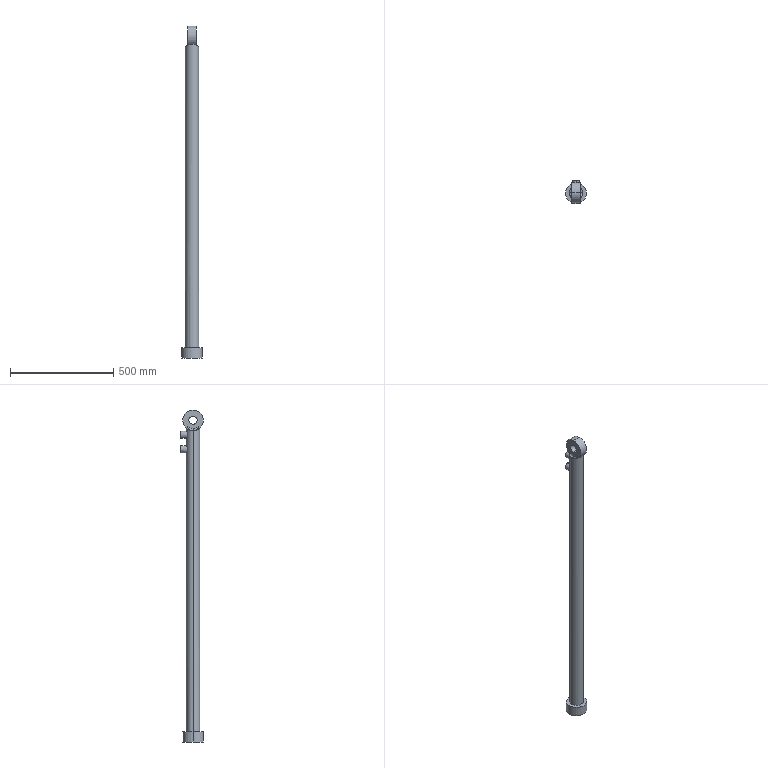Part | SolidWorks | features ICE 5, Fillet 2, Extrusion 1 | 1 solid | 30 faces | box 100 x 110 x 1610 mm | volume 5542883 mm3 | cylinder 18 | plane 8 | torus 4 | commonest cylinder face diameters 100 x6 20 x4 35 x4 40 x2 65 x2
STEP:
#1=CARTESIAN_POINT('',(0.,20.,1360.));
#2=VERTEX_POINT('',#1);
#3=CARTESIAN_POINT('',(0.,20.,1380.));
#4=VERTEX_POINT('',#3);
#5=CARTESIAN_POINT('',(0.,20.,1370.));
#6=DIRECTION('',(0.,1.,0.));
#7=DIRECTION('',(0.,0.,1.));
#8=AXIS2_PLACEMENT_3D('',#5,#6,#7);
#9=CIRCLE('',#8,10.);
#10=EDGE_CURVE('',#2,#4,#9,.T.);
#11=ORIENTED_EDGE('',*,*,#10,.F.);
#12=CARTESIAN_POINT('',(0.,60.,1360.));
#13=VERTEX_POINT('',#12);
#14=CARTESIAN_POINT('',(0.,20.,1360.));
#15=DIRECTION('',(0.,1.,0.));
#16=VECTOR('',#15,1000.);
#17=LINE('',#14,#16);
#18=EDGE_CURVE('',#2,#13,#17,.T.);
#19=ORIENTED_EDGE('',*,*,#18,.T.);
#20=CARTESIAN_POINT('',(0.,60.,1380.));
#21=VERTEX_POINT('',#20);
#22=CARTESIAN_POINT('',(0.,60.,1370.));
#23=DIRECTION('',(0.,1.,0.));
#24=DIRECTION('',(0.,0.,1.));
#25=AXIS2_PLACEMENT_3D('',#22,#23,#24);
#26=CIRCLE('',#25,10.);
#27=EDGE_CURVE('',#13,#21,#26,.T.);
#28=ORIENTED_EDGE('',*,*,#27,.T.);
#29=CARTESIAN_POINT('',(0.,20.,1380.));
#30=DIRECTION('',(0.,1.,0.));
#31=VECTOR('',#30,1000.);
#32=LINE('',#29,#31);
#33=EDGE_CURVE('',#4,#21,#32,.T.);
#34=ORIENTED_EDGE('',*,*,#33,.F.);
#35=EDGE_LOOP('',(#11,#19,#28,#34));
#36=FACE_OUTER_BOUND('',#35,.T.);
#37=CARTESIAN_POINT('',(0.,20.,1370.));
#38=DIRECTION('',(0.,1.,0.));
#39=DIRECTION('',(0.,0.,1.));
#40=AXIS2_PLACEMENT_3D('',#37,#38,#39);
#41=CYLINDRICAL_SURFACE('',#40,10.);
#42=ADVANCED_FACE('',(#36),#41,.F.);
#43=CARTESIAN_POINT('',(0.,20.,1430.));
#44=VERTEX_POINT('',#43);
#45=CARTESIAN_POINT('',(0.,20.,1450.));
#46=VERTEX_POINT('',#45);
#47=CARTESIAN_POINT('',(0.,20.,1440.));
#48=DIRECTION('',(0.,1.,0.));
#49=DIRECTION('',(0.,0.,1.));
#50=AXIS2_PLACEMENT_3D('',#47,#48,#49);
#51=CIRCLE('',#50,10.);
#52=EDGE_CURVE('',#44,#46,#51,.T.);
#53=ORIENTED_EDGE('',*,*,#52,.F.);
#54=CARTESIAN_POINT('',(0.,60.,1430.));
#55=VERTEX_POINT('',#54);
#56=CARTESIAN_POINT('',(0.,20.,1430.));
#57=DIRECTION('',(0.,1.,0.));
#58=VECTOR('',#57,1000.);
#59=LINE('',#56,#58);
#60=EDGE_CURVE('',#44,#55,#59,.T.);
#61=ORIENTED_EDGE('',*,*,#60,.T.);
#62=CARTESIAN_POINT('',(0.,60.,1450.));
#63=VERTEX_POINT('',#62);
#64=CARTESIAN_POINT('',(0.,60.,1440.));
#65=DIRECTION('',(0.,1.,0.));
#66=DIRECTION('',(0.,0.,1.));
#67=AXIS2_PLACEMENT_3D('',#64,#65,#66);
#68=CIRCLE('',#67,10.);
#69=EDGE_CURVE('',#55,#63,#68,.T.);
#70=ORIENTED_EDGE('',*,*,#69,.T.);
#71=CARTESIAN_POINT('',(0.,20.,1450.));
#72=DIRECTION('',(0.,1.,0.));
#73=VECTOR('',#72,1000.);
#74=LINE('',#71,#73);
#75=EDGE_CURVE('',#46,#63,#74,.T.);
#76=ORIENTED_EDGE('',*,*,#75,.F.);
#77=EDGE_LOOP('',(#53,#61,#70,#76));
#78=FACE_OUTER_BOUND('',#77,.T.);
#79=CARTESIAN_POINT('',(0.,20.,1440.));
#80=DIRECTION('',(0.,1.,0.));
#81=DIRECTION('',(0.,0.,1.));
#82=AXIS2_PLACEMENT_3D('',#79,#80,#81);
#83=CYLINDRICAL_SURFACE('',#82,10.);
#84=ADVANCED_FACE('',(#78),#83,.F.);
#85=CARTESIAN_POINT('',(0.,32.5,1387.5));
#86=VERTEX_POINT('',#85);
#87=CARTESIAN_POINT('',(0.,32.5,1352.5));
#88=VERTEX_POINT('',#87);
#89=CARTESIAN_POINT('',(0.,32.5,1387.5));
#90=CARTESIAN_POINT('',(1.182,32.5,1387.5));
#91=CARTESIAN_POINT('',(2.339,32.436,1387.382));
#92=CARTESIAN_POINT('',(4.042,32.253,1387.037));
#93=CARTESIAN_POINT('',(4.604,32.177,1386.893));
#94=CARTESIAN_POINT('',(5.717,31.998,1386.55));
#95=CARTESIAN_POINT('',(6.262,31.896,1386.351));
#96=CARTESIAN_POINT('',(7.847,31.557,1385.684));
#97=CARTESIAN_POINT('',(8.845,31.289,1385.143));
#98=CARTESIAN_POINT('',(10.259,30.842,1384.189));
#99=CARTESIAN_POINT('',(10.715,30.686,1383.848));
#100=CARTESIAN_POINT('',(11.583,30.369,1383.13));
#101=CARTESIAN_POINT('',(11.997,30.208,1382.753));
#102=CARTESIAN_POINT('',(12.787,29.882,1381.961));
#103=CARTESIAN_POINT('',(13.163,29.718,1381.545));
#104=CARTESIAN_POINT('',(13.878,29.391,1380.676));
#105=CARTESIAN_POINT('',(14.217,29.227,1380.22));
#106=CARTESIAN_POINT('',(15.16,28.756,1378.814));
#107=CARTESIAN_POINT('',(15.695,28.464,1377.824));
#108=CARTESIAN_POINT('',(16.354,28.086,1376.253));
#109=CARTESIAN_POINT('',(16.551,27.971,1375.715));
#110=CARTESIAN_POINT('',(16.807,27.817,1374.884));
#111=CARTESIAN_POINT('',(16.886,27.769,1374.603));
#112=CARTESIAN_POINT('',(17.03,27.681,1374.041));
#113=CARTESIAN_POINT('',(17.094,27.641,1373.758));
#114=CARTESIAN_POINT('',(17.381,27.463,1372.341));
#115=CARTESIAN_POINT('',(17.499,27.387,1371.19));
#116=CARTESIAN_POINT('',(17.501,27.386,1369.437));
#117=CARTESIAN_POINT('',(17.472,27.404,1368.843));
#118=CARTESIAN_POINT('',(17.355,27.478,1367.677));
#119=CARTESIAN_POINT('',(17.268,27.533,1367.102));
#120=CARTESIAN_POINT('',(17.039,27.676,1365.967));
#121=CARTESIAN_POINT('',(16.897,27.763,1365.408));
#122=CARTESIAN_POINT('',(16.557,27.967,1364.303));
#123=CARTESIAN_POINT('',(16.358,28.084,1363.757));
#124=CARTESIAN_POINT('',(15.693,28.465,1362.171));
#125=CARTESIAN_POINT('',(15.155,28.759,1361.177));
#126=CARTESIAN_POINT('',(14.208,29.232,1359.768));
#127=CARTESIAN_POINT('',(13.868,29.395,1359.312));
#128=CARTESIAN_POINT('',(13.153,29.722,1358.442));
#129=CARTESIAN_POINT('',(12.776,29.887,1358.028));
#130=CARTESIAN_POINT('',(11.985,30.213,1357.236));
#131=CARTESIAN_POINT('',(11.57,30.374,1356.859));
#132=CARTESIAN_POINT('',(10.702,30.691,1356.142));
#133=CARTESIAN_POINT('',(10.247,30.846,1355.802));
#134=CARTESIAN_POINT('',(8.828,31.294,1354.847));
#135=CARTESIAN_POINT('',(7.831,31.561,1354.308));
#136=CARTESIAN_POINT('',(6.255,31.897,1353.646));
#137=CARTESIAN_POINT('',(5.716,31.998,1353.45));
#138=CARTESIAN_POINT('',(4.609,32.176,1353.108));
#139=CARTESIAN_POINT('',(4.038,32.253,1352.962));
#140=CARTESIAN_POINT('',(2.323,32.437,1352.616));
#141=CARTESIAN_POINT('',(1.168,32.5,1352.5));
#142=CARTESIAN_POINT('',(0.,32.5,1352.5));
#143=B_SPLINE_CURVE_WITH_KNOTS('',3,(#89,#90,#91,#92,#93,#94,#95,#96,#97,#98,#99,#100,#101,#102,#103,#104,#105,#106,#107,#108,#109,#110,#111,#112,#113,#114,#115,#116,#117,#118,#119,#120,#121,#122,#123,#124,#125,#126,#127,#128,#129,#130,#131,#132,#133,#134,#135,#136,#137,#138,#139,#140,#141,#142),.UNSPECIFIED.,.F.,.F.,(4,2,2,2,2,2,2,2,2,2,2,2,2,2,2,2,2,2,2,2,2,2,2,2,2,2,4),(0.,0.00349,0.005235,0.00698,0.01047,0.01222,0.01396,0.01571,0.01745,0.02094,0.02269,0.02356,0.02443,0.02792,0.02967,0.03141,0.03316,0.0349,0.03839,0.04014,0.04188,0.04363,0.04537,0.04886,0.05061,0.05235,0.05584),.UNSPECIFIED.);
#144=EDGE_CURVE('',#86,#88,#143,.T.);
#145=ORIENTED_EDGE('',*,*,#144,.T.);
#146=CARTESIAN_POINT('',(0.,60.,1352.5));
#147=VERTEX_POINT('',#146);
#148=CARTESIAN_POINT('',(0.,-50.001,1352.5));
#149=DIRECTION('',(0.,1.,0.));
#150=VECTOR('',#149,1000.);
#151=LINE('',#148,#150);
#152=EDGE_CURVE('',#88,#147,#151,.T.);
#153=ORIENTED_EDGE('',*,*,#152,.T.);
#154=CARTESIAN_POINT('',(0.,60.,1387.5));
#155=VERTEX_POINT('',#154);
#156=CARTESIAN_POINT('',(0.,60.,1370.));
#157=DIRECTION('',(0.,1.,0.));
#158=DIRECTION('',(0.,0.,1.));
#159=AXIS2_PLACEMENT_3D('',#156,#157,#158);
#160=CIRCLE('',#159,17.5);
#161=EDGE_CURVE('',#155,#147,#160,.T.);
#162=ORIENTED_EDGE('',*,*,#161,.F.);
#163=CARTESIAN_POINT('',(0.,-50.001,1387.5));
#164=DIRECTION('',(0.,1.,0.));
#165=VECTOR('',#164,1000.);
#166=LINE('',#163,#165);
#167=EDGE_CURVE('',#86,#155,#166,.T.);
#168=ORIENTED_EDGE('',*,*,#167,.F.);
#169=EDGE_LOOP('',(#145,#153,#162,#168));
#170=FACE_OUTER_BOUND('',#169,.T.);
#171=CARTESIAN_POINT('',(0.,-50.001,1370.));
#172=DIRECTION('',(0.,1.,0.));
#173=DIRECTION('',(0.,0.,1.));
#174=AXIS2_PLACEMENT_3D('',#171,#172,#173);
#175=CYLINDRICAL_SURFACE('',#174,17.5);
#176=ADVANCED_FACE('',(#170),#175,.T.);
#177=CARTESIAN_POINT('',(0.,32.5,1457.5));
#178=VERTEX_POINT('',#177);
#179=CARTESIAN_POINT('',(0.,32.5,1422.5));
#180=VERTEX_POINT('',#179);
#181=CARTESIAN_POINT('',(0.,32.5,1457.5));
#182=CARTESIAN_POINT('',(1.182,32.5,1457.5));
#183=CARTESIAN_POINT('',(2.339,32.436,1457.382));
#184=CARTESIAN_POINT('',(4.042,32.253,1457.037));
#185=CARTESIAN_POINT('',(4.604,32.177,1456.893));
#186=CARTESIAN_POINT('',(5.717,31.998,1456.55));
#187=CARTESIAN_POINT('',(6.262,31.896,1456.351));
#188=CARTESIAN_POINT('',(7.847,31.557,1455.684));
#189=CARTESIAN_POINT('',(8.845,31.289,1455.143));
#190=CARTESIAN_POINT('',(10.259,30.842,1454.189));
#191=CARTESIAN_POINT('',(10.715,30.686,1453.848));
#192=CARTESIAN_POINT('',(11.583,30.369,1453.13));
#193=CARTESIAN_POINT('',(11.997,30.208,1452.753));
#194=CARTESIAN_POINT('',(12.787,29.882,1451.961));
#195=CARTESIAN_POINT('',(13.163,29.718,1451.545));
#196=CARTESIAN_POINT('',(13.878,29.391,1450.676));
#197=CARTESIAN_POINT('',(14.217,29.227,1450.22));
#198=CARTESIAN_POINT('',(15.16,28.756,1448.814));
#199=CARTESIAN_POINT('',(15.695,28.464,1447.824));
#200=CARTESIAN_POINT('',(16.354,28.086,1446.253));
#201=CARTESIAN_POINT('',(16.551,27.971,1445.715));
#202=CARTESIAN_POINT('',(16.807,27.817,1444.884));
#203=CARTESIAN_POINT('',(16.886,27.769,1444.603));
#204=CARTESIAN_POINT('',(17.03,27.681,1444.041));
#205=CARTESIAN_POINT('',(17.094,27.641,1443.758));
#206=CARTESIAN_POINT('',(17.381,27.463,1442.341));
#207=CARTESIAN_POINT('',(17.499,27.387,1441.19));
#208=CARTESIAN_POINT('',(17.501,27.386,1439.437));
#209=CARTESIAN_POINT('',(17.472,27.404,1438.843));
#210=CARTESIAN_POINT('',(17.355,27.478,1437.677));
#211=CARTESIAN_POINT('',(17.268,27.533,1437.102));
#212=CARTESIAN_POINT('',(17.039,27.676,1435.967));
#213=CARTESIAN_POINT('',(16.897,27.763,1435.408));
#214=CARTESIAN_POINT('',(16.557,27.967,1434.303));
#215=CARTESIAN_POINT('',(16.358,28.084,1433.757));
#216=CARTESIAN_POINT('',(15.693,28.465,1432.171));
#217=CARTESIAN_POINT('',(15.155,28.759,1431.177));
#218=CARTESIAN_POINT('',(14.208,29.232,1429.768));
#219=CARTESIAN_POINT('',(13.868,29.395,1429.312));
#220=CARTESIAN_POINT('',(13.153,29.722,1428.442));
#221=CARTESIAN_POINT('',(12.776,29.887,1428.028));
#222=CARTESIAN_POINT('',(11.985,30.213,1427.236));
#223=CARTESIAN_POINT('',(11.57,30.374,1426.859));
#224=CARTESIAN_POINT('',(10.702,30.691,1426.142));
#225=CARTESIAN_POINT('',(10.247,30.846,1425.802));
#226=CARTESIAN_POINT('',(8.828,31.294,1424.847));
#227=CARTESIAN_POINT('',(7.831,31.561,1424.308));
#228=CARTESIAN_POINT('',(6.255,31.897,1423.646));
#229=CARTESIAN_POINT('',(5.716,31.998,1423.45));
#230=CARTESIAN_POINT('',(4.609,32.176,1423.108));
#231=CARTESIAN_POINT('',(4.038,32.253,1422.962));
#232=CARTESIAN_POINT('',(2.323,32.437,1422.616));
#233=CARTESIAN_POINT('',(1.168,32.5,1422.5));
#234=CARTESIAN_POINT('',(0.,32.5,1422.5));
#235=B_SPLINE_CURVE_WITH_KNOTS('',3,(#181,#182,#183,#184,#185,#186,#187,#188,#189,#190,#191,#192,#193,#194,#195,#196,#197,#198,#199,#200,#201,#202,#203,#204,#205,#206,#207,#208,#209,#210,#211,#212,#213,#214,#215,#216,#217,#218,#219,#220,#221,#222,#223,#224,#225,#226,#227,#228,#229,#230,#231,#232,#233,#234),.UNSPECIFIED.,.F.,.F.,(4,2,2,2,2,2,2,2,2,2,2,2,2,2,2,2,2,2,2,2,2,2,2,2,2,2,4),(0.,0.00349,0.005235,0.00698,0.01047,0.01222,0.01396,0.01571,0.01745,0.02094,0.02269,0.02356,0.02443,0.02792,0.02967,0.03141,0.03316,0.0349,0.03839,0.04014,0.04188,0.04363,0.04537,0.04886,0.05061,0.05235,0.05584),.UNSPECIFIED.);
#236=EDGE_CURVE('',#178,#180,#235,.T.);
#237=ORIENTED_EDGE('',*,*,#236,.T.);
#238=CARTESIAN_POINT('',(0.,60.,1422.5));
#239=VERTEX_POINT('',#238);
#240=CARTESIAN_POINT('',(0.,-50.001,1422.5));
#241=DIRECTION('',(0.,1.,0.));
#242=VECTOR('',#241,1000.);
#243=LINE('',#240,#242);
#244=EDGE_CURVE('',#180,#239,#243,.T.);
#245=ORIENTED_EDGE('',*,*,#244,.T.);
#246=CARTESIAN_POINT('',(0.,60.,1457.5));
#247=VERTEX_POINT('',#246);
#248=CARTESIAN_POINT('',(0.,60.,1440.));
#249=DIRECTION('',(0.,1.,0.));
#250=DIRECTION('',(0.,0.,1.));
#251=AXIS2_PLACEMENT_3D('',#248,#249,#250);
#252=CIRCLE('',#251,17.5);
#253=EDGE_CURVE('',#247,#239,#252,.T.);
#254=ORIENTED_EDGE('',*,*,#253,.F.);
#255=CARTESIAN_POINT('',(0.,-50.001,1457.5));
#256=DIRECTION('',(0.,1.,0.));
#257=VECTOR('',#256,1000.);
#258=LINE('',#255,#257);
#259=EDGE_CURVE('',#178,#247,#258,.T.);
#260=ORIENTED_EDGE('',*,*,#259,.F.);
#261=EDGE_LOOP('',(#237,#245,#254,#260));
#262=FACE_OUTER_BOUND('',#261,.T.);
#263=CARTESIAN_POINT('',(0.,-50.001,1440.));
#264=DIRECTION('',(0.,1.,0.));
#265=DIRECTION('',(0.,0.,1.));
#266=AXIS2_PLACEMENT_3D('',#263,#264,#265);
#267=CYLINDRICAL_SURFACE('',#266,17.5);
#268=ADVANCED_FACE('',(#262),#267,.T.);
#269=CARTESIAN_POINT('',(20.,0.,1470.));
#270=VERTEX_POINT('',#269);
#271=CARTESIAN_POINT('',(20.,25.617,1479.279));
#272=VERTEX_POINT('',#271);
#273=CARTESIAN_POINT('',(20.,0.,1510.));
#274=DIRECTION('',(1.,0.,0.));
#275=DIRECTION('',(0.,0.,-1.));
#276=AXIS2_PLACEMENT_3D('',#273,#274,#275);
#277=CIRCLE('',#276,40.);
#278=EDGE_CURVE('',#270,#272,#277,.T.);
#279=ORIENTED_EDGE('',*,*,#278,.F.);
#280=CARTESIAN_POINT('',(30.,0.,1460.));
#281=VERTEX_POINT('',#280);
#282=CARTESIAN_POINT('',(30.,0.,1470.));
#283=DIRECTION('',(0.,-1.,0.));
#284=DIRECTION('',(0.,0.,-1.));
#285=AXIS2_PLACEMENT_3D('',#282,#283,#284);
#286=CIRCLE('',#285,10.);
#287=EDGE_CURVE('',#270,#281,#286,.T.);
#288=ORIENTED_EDGE('',*,*,#287,.T.);
#289=CARTESIAN_POINT('',(30.,12.5,1461.588));
#290=VERTEX_POINT('',#289);
#291=CARTESIAN_POINT('',(30.,0.,1510.));
#292=DIRECTION('',(-1.,0.,0.));
#293=DIRECTION('',(0.,0.,-1.));
#294=AXIS2_PLACEMENT_3D('',#291,#292,#293);
#295=CIRCLE('',#294,50.);
#296=EDGE_CURVE('',#290,#281,#295,.T.);
#297=ORIENTED_EDGE('',*,*,#296,.F.);
#298=CARTESIAN_POINT('',(20.,25.617,1479.279));
#299=CARTESIAN_POINT('',(20.,25.617,1478.174));
#300=CARTESIAN_POINT('',(20.105,25.536,1477.092));
#301=CARTESIAN_POINT('',(20.389,25.309,1475.497));
#302=CARTESIAN_POINT('',(20.504,25.216,1474.971));
#303=CARTESIAN_POINT('',(20.777,24.992,1473.927));
#304=CARTESIAN_POINT('',(20.932,24.863,1473.415));
#305=CARTESIAN_POINT('',(21.445,24.425,1471.921));
#306=CARTESIAN_POINT('',(21.852,24.065,1470.974));
#307=CARTESIAN_POINT('',(22.542,23.414,1469.624));
#308=CARTESIAN_POINT('',(22.785,23.178,1469.188));
#309=CARTESIAN_POINT('',(23.284,22.677,1468.355));
#310=CARTESIAN_POINT('',(23.541,22.41,1467.956));
#311=CARTESIAN_POINT('',(24.068,21.843,1467.191));
#312=CARTESIAN_POINT('',(24.338,21.542,1466.825));
#313=CARTESIAN_POINT('',(24.887,20.906,1466.124));
#314=CARTESIAN_POINT('',(25.167,20.569,1465.789));
#315=CARTESIAN_POINT('',(26.004,19.515,1464.839));
#316=CARTESIAN_POINT('',(26.558,18.758,1464.284));
#317=CARTESIAN_POINT('',(27.364,17.541,1463.549));
#318=CARTESIAN_POINT('',(27.629,17.122,1463.32));
#319=CARTESIAN_POINT('',(28.147,16.256,1462.893));
#320=CARTESIAN_POINT('',(28.401,15.808,1462.695));
#321=CARTESIAN_POINT('',(29.135,14.439,1462.147));
#322=CARTESIAN_POINT('',(29.588,13.488,1461.843));
#323=CARTESIAN_POINT('',(30.,12.5,1461.588));
#324=B_SPLINE_CURVE_WITH_KNOTS('',3,(#298,#299,#300,#301,#302,#303,#304,#305,#306,#307,#308,#309,#310,#311,#312,#313,#314,#315,#316,#317,#318,#319,#320,#321,#322,#323),.UNSPECIFIED.,.F.,.F.,(4,2,2,2,2,2,2,2,2,2,2,2,4),(0.,0.003267,0.0049,0.006533,0.0098,0.01143,0.01307,0.0147,0.01633,0.0196,0.02123,0.02287,0.02613),.UNSPECIFIED.);
#325=EDGE_CURVE('',#272,#290,#324,.T.);
#326=ORIENTED_EDGE('',*,*,#325,.F.);
#327=EDGE_LOOP('',(#279,#288,#297,#326));
#328=FACE_OUTER_BOUND('',#327,.T.);
#329=CARTESIAN_POINT('',(30.,0.,1510.));
#330=DIRECTION('',(1.,0.,0.));
#331=DIRECTION('',(0.,0.,-1.));
#332=AXIS2_PLACEMENT_3D('',#329,#330,#331);
#333=TOROIDAL_SURFACE('',#332,40.,10.);
#334=ADVANCED_FACE('',(#328),#333,.F.);
#335=CARTESIAN_POINT('',(-30.,0.,1460.));
#336=VERTEX_POINT('',#335);
#337=CARTESIAN_POINT('',(-30.,12.5,1461.588));
#338=VERTEX_POINT('',#337);
#339=CARTESIAN_POINT('',(-30.,0.,1510.));
#340=DIRECTION('',(1.,0.,0.));
#341=DIRECTION('',(0.,0.,-1.));
#342=AXIS2_PLACEMENT_3D('',#339,#340,#341);
#343=CIRCLE('',#342,50.);
#344=EDGE_CURVE('',#336,#338,#343,.T.);
#345=ORIENTED_EDGE('',*,*,#344,.F.);
#346=CARTESIAN_POINT('',(-20.,0.,1470.));
#347=VERTEX_POINT('',#346);
#348=CARTESIAN_POINT('',(-30.,0.,1470.));
#349=DIRECTION('',(0.,-1.,0.));
#350=DIRECTION('',(0.,0.,-1.));
#351=AXIS2_PLACEMENT_3D('',#348,#349,#350);
#352=CIRCLE('',#351,10.);
#353=EDGE_CURVE('',#336,#347,#352,.T.);
#354=ORIENTED_EDGE('',*,*,#353,.T.);
#355=CARTESIAN_POINT('',(-20.,25.617,1479.279));
#356=VERTEX_POINT('',#355);
#357=CARTESIAN_POINT('',(-20.,0.,1510.));
#358=DIRECTION('',(-1.,0.,0.));
#359=DIRECTION('',(0.,0.,-1.));
#360=AXIS2_PLACEMENT_3D('',#357,#358,#359);
#361=CIRCLE('',#360,40.);
#362=EDGE_CURVE('',#356,#347,#361,.T.);
#363=ORIENTED_EDGE('',*,*,#362,.F.);
#364=CARTESIAN_POINT('',(-30.,12.5,1461.588));
#365=CARTESIAN_POINT('',(-29.175,14.481,1462.099));
#366=CARTESIAN_POINT('',(-28.19,16.291,1462.798));
#367=CARTESIAN_POINT('',(-26.84,18.333,1464.027));
#368=CARTESIAN_POINT('',(-26.563,18.732,1464.292));
#369=CARTESIAN_POINT('',(-26.006,19.498,1464.856));
#370=CARTESIAN_POINT('',(-25.727,19.863,1465.153));
#371=CARTESIAN_POINT('',(-24.894,20.912,1466.097));
#372=CARTESIAN_POINT('',(-24.344,21.547,1466.792));
#373=CARTESIAN_POINT('',(-23.546,22.406,1467.949));
#374=CARTESIAN_POINT('',(-23.283,22.678,1468.356));
#375=CARTESIAN_POINT('',(-22.781,23.182,1469.194));
#376=CARTESIAN_POINT('',(-22.541,23.415,1469.626));
#377=CARTESIAN_POINT('',(-21.857,24.06,1470.963));
#378=CARTESIAN_POINT('',(-21.45,24.42,1471.908));
#379=CARTESIAN_POINT('',(-20.933,24.862,1473.41));
#380=CARTESIAN_POINT('',(-20.777,24.992,1473.927));
#381=CARTESIAN_POINT('',(-20.505,25.215,1474.967));
#382=CARTESIAN_POINT('',(-20.39,25.309,1475.493));
#383=CARTESIAN_POINT('',(-20.106,25.535,1477.086));
#384=CARTESIAN_POINT('',(-20.,25.617,1478.169));
#385=CARTESIAN_POINT('',(-20.,25.617,1479.279));
#386=B_SPLINE_CURVE_WITH_KNOTS('',3,(#364,#365,#366,#367,#368,#369,#370,#371,#372,#373,#374,#375,#376,#377,#378,#379,#380,#381,#382,#383,#384,#385),.UNSPECIFIED.,.F.,.F.,(4,2,2,2,2,2,2,2,2,2,4),(0.,0.006524,0.008155,0.009786,0.01305,0.01468,0.01631,0.01957,0.0212,0.02283,0.0261),.UNSPECIFIED.);
#387=EDGE_CURVE('',#338,#356,#386,.T.);
#388=ORIENTED_EDGE('',*,*,#387,.F.);
#389=EDGE_LOOP('',(#345,#354,#363,#388));
#390=FACE_OUTER_BOUND('',#389,.T.);
#391=CARTESIAN_POINT('',(-30.,0.,1510.));
#392=DIRECTION('',(1.,0.,0.));
#393=DIRECTION('',(0.,0.,-1.));
#394=AXIS2_PLACEMENT_3D('',#391,#392,#393);
#395=TOROIDAL_SURFACE('',#394,40.,10.);
#396=ADVANCED_FACE('',(#390),#395,.F.);
#397=CARTESIAN_POINT('',(20.,0.,1530.));
#398=VERTEX_POINT('',#397);
#399=CARTESIAN_POINT('',(20.,0.,1490.));
#400=VERTEX_POINT('',#399);
#401=CARTESIAN_POINT('',(20.,0.,1510.));
#402=DIRECTION('',(1.,0.,0.));
#403=DIRECTION('',(0.,0.,-1.));
#404=AXIS2_PLACEMENT_3D('',#401,#402,#403);
#405=CIRCLE('',#404,20.);
#406=EDGE_CURVE('',#398,#400,#405,.T.);
#407=ORIENTED_EDGE('',*,*,#406,.T.);
#408=CARTESIAN_POINT('',(-20.,0.,1490.));
#409=VERTEX_POINT('',#408);
#410=CARTESIAN_POINT('',(20.,0.,1490.));
#411=DIRECTION('',(-1.,0.,0.));
#412=VECTOR('',#411,1000.);
#413=LINE('',#410,#412);
#414=EDGE_CURVE('',#400,#409,#413,.T.);
#415=ORIENTED_EDGE('',*,*,#414,.T.);
#416=CARTESIAN_POINT('',(-20.,0.,1530.));
#417=VERTEX_POINT('',#416);
#418=CARTESIAN_POINT('',(-20.,0.,1510.));
#419=DIRECTION('',(1.,0.,0.));
#420=DIRECTION('',(0.,0.,-1.));
#421=AXIS2_PLACEMENT_3D('',#418,#419,#420);
#422=CIRCLE('',#421,20.);
#423=EDGE_CURVE('',#417,#409,#422,.T.);
#424=ORIENTED_EDGE('',*,*,#423,.F.);
#425=CARTESIAN_POINT('',(20.,0.,1530.));
#426=DIRECTION('',(-1.,0.,0.));
#427=VECTOR('',#426,1000.);
#428=LINE('',#425,#427);
#429=EDGE_CURVE('',#398,#417,#428,.T.);
#430=ORIENTED_EDGE('',*,*,#429,.F.);
#431=EDGE_LOOP('',(#407,#415,#424,#430));
#432=FACE_OUTER_BOUND('',#431,.T.);
#433=CARTESIAN_POINT('',(20.,0.,1510.));
#434=DIRECTION('',(-1.,0.,0.));
#435=DIRECTION('',(0.,0.,1.));
#436=AXIS2_PLACEMENT_3D('',#433,#434,#435);
#437=CYLINDRICAL_SURFACE('',#436,20.);
#438=ADVANCED_FACE('',(#432),#437,.F.);
#439=CARTESIAN_POINT('',(20.,0.,1560.));
#440=VERTEX_POINT('',#439);
#441=CARTESIAN_POINT('',(20.,-25.617,1467.061));
#442=VERTEX_POINT('',#441);
#443=CARTESIAN_POINT('',(20.,0.,1510.));
#444=DIRECTION('',(1.,0.,0.));
#445=DIRECTION('',(0.,0.,-1.));
#446=AXIS2_PLACEMENT_3D('',#443,#444,#445);
#447=CIRCLE('',#446,50.);
#448=EDGE_CURVE('',#440,#442,#447,.T.);
#449=ORIENTED_EDGE('',*,*,#448,.F.);
#450=CARTESIAN_POINT('',(-20.,0.,1560.));
#451=VERTEX_POINT('',#450);
#452=CARTESIAN_POINT('',(20.,0.,1560.));
#453=DIRECTION('',(-1.,0.,0.));
#454=VECTOR('',#453,1000.);
#455=LINE('',#452,#454);
#456=EDGE_CURVE('',#440,#451,#455,.T.);
#457=ORIENTED_EDGE('',*,*,#456,.T.);
#458=CARTESIAN_POINT('',(-20.,-25.617,1467.061));
#459=VERTEX_POINT('',#458);
#460=CARTESIAN_POINT('',(-20.,0.,1510.));
#461=DIRECTION('',(1.,0.,0.));
#462=DIRECTION('',(0.,0.,-1.));
#463=AXIS2_PLACEMENT_3D('',#460,#461,#462);
#464=CIRCLE('',#463,50.);
#465=EDGE_CURVE('',#451,#459,#464,.T.);
#466=ORIENTED_EDGE('',*,*,#465,.T.);
#467=CARTESIAN_POINT('',(-20.,-25.617,1467.061));
#468=CARTESIAN_POINT('',(-18.622,-26.693,1467.703));
#469=CARTESIAN_POINT('',(-17.172,-27.648,1468.327));
#470=CARTESIAN_POINT('',(-14.117,-29.325,1469.49));
#471=CARTESIAN_POINT('',(-12.513,-30.049,1470.029));
#472=CARTESIAN_POINT('',(-10.39,-30.798,1470.61));
#473=CARTESIAN_POINT('',(-9.958,-30.94,1470.722));
#474=CARTESIAN_POINT('',(-9.09,-31.206,1470.933));
#475=CARTESIAN_POINT('',(-8.654,-31.33,1471.033));
#476=CARTESIAN_POINT('',(-7.336,-31.674,1471.311));
#477=CARTESIAN_POINT('',(-6.447,-31.867,1471.471));
#478=CARTESIAN_POINT('',(-4.646,-32.179,1471.731));
#479=CARTESIAN_POINT('',(-3.735,-32.298,1471.831));
#480=CARTESIAN_POINT('',(-1.889,-32.458,1471.967));
#481=CARTESIAN_POINT('',(-0.9499,-32.499,1472.003));
#482=CARTESIAN_POINT('',(1.835,-32.501,1472.004));
#483=CARTESIAN_POINT('',(3.667,-32.345,1471.869));
#484=CARTESIAN_POINT('',(5.928,-31.958,1471.546));
#485=CARTESIAN_POINT('',(6.378,-31.871,1471.474));
#486=CARTESIAN_POINT('',(7.277,-31.678,1471.315));
#487=CARTESIAN_POINT('',(7.725,-31.572,1471.228));
#488=CARTESIAN_POINT('',(9.05,-31.228,1470.95));
#489=CARTESIAN_POINT('',(9.913,-30.964,1470.74));
#490=CARTESIAN_POINT('',(11.605,-30.371,1470.279));
#491=CARTESIAN_POINT('',(12.433,-30.041,1470.028));
#492=CARTESIAN_POINT('',(14.057,-29.316,1469.494));
#493=CARTESIAN_POINT('',(14.855,-28.92,1469.209));
#494=CARTESIAN_POINT('',(17.178,-27.646,1468.325));
#495=CARTESIAN_POINT('',(18.631,-26.686,1467.699));
#496=CARTESIAN_POINT('',(20.,-25.617,1467.061));
#497=B_SPLINE_CURVE_WITH_KNOTS('',3,(#467,#468,#469,#470,#471,#472,#473,#474,#475,#476,#477,#478,#479,#480,#481,#482,#483,#484,#485,#486,#487,#488,#489,#490,#491,#492,#493,#494,#495,#496),.UNSPECIFIED.,.F.,.F.,(4,2,2,2,2,2,2,2,2,2,2,2,2,2,4),(0.03034,0.03586,0.04138,0.04276,0.04414,0.0469,0.04966,0.05242,0.05794,0.05932,0.0607,0.06346,0.06622,0.06898,0.0745),.UNSPECIFIED.);
#498=EDGE_CURVE('',#459,#442,#497,.T.);
#499=ORIENTED_EDGE('',*,*,#498,.T.);
#500=EDGE_LOOP('',(#449,#457,#466,#499));
#501=FACE_OUTER_BOUND('',#500,.T.);
#502=CARTESIAN_POINT('',(20.,0.,1510.));
#503=DIRECTION('',(-1.,0.,0.));
#504=DIRECTION('',(0.,0.,1.));
#505=AXIS2_PLACEMENT_3D('',#502,#503,#504);
#506=CYLINDRICAL_SURFACE('',#505,50.);
#507=ADVANCED_FACE('',(#501),#506,.T.);
#508=CARTESIAN_POINT('',(-50.,0.,-50.));
#509=VERTEX_POINT('',#508);
#510=CARTESIAN_POINT('',(50.,0.,-50.));
#511=VERTEX_POINT('',#510);
#512=CARTESIAN_POINT('',(0.,0.,-50.));
#513=DIRECTION('',(0.,0.,-1.));
#514=DIRECTION('',(-1.,0.,0.));
#515=AXIS2_PLACEMENT_3D('',#512,#513,#514);
#516=CIRCLE('',#515,50.);
#517=EDGE_CURVE('',#509,#511,#516,.T.);
#518=ORIENTED_EDGE('',*,*,#517,.F.);
#519=CARTESIAN_POINT('',(-50.,0.,0.));
#520=VERTEX_POINT('',#519);
#521=CARTESIAN_POINT('',(-50.,0.,-50.));
#522=DIRECTION('',(0.,0.,1.));
#523=VECTOR('',#522,1000.);
#524=LINE('',#521,#523);
#525=EDGE_CURVE('',#509,#520,#524,.T.);
#526=ORIENTED_EDGE('',*,*,#525,.T.);
#527=CARTESIAN_POINT('',(50.,0.,0.));
#528=VERTEX_POINT('',#527);
#529=CARTESIAN_POINT('',(0.,0.,0.));
#530=DIRECTION('',(0.,0.,-1.));
#531=DIRECTION('',(-1.,0.,0.));
#532=AXIS2_PLACEMENT_3D('',#529,#530,#531);
#533=CIRCLE('',#532,50.);
#534=EDGE_CURVE('',#520,#528,#533,.T.);
#535=ORIENTED_EDGE('',*,*,#534,.T.);
#536=CARTESIAN_POINT('',(50.,0.,-50.));
#537=DIRECTION('',(0.,0.,1.));
#538=VECTOR('',#537,1000.);
#539=LINE('',#536,#538);
#540=EDGE_CURVE('',#511,#528,#539,.T.);
#541=ORIENTED_EDGE('',*,*,#540,.F.);
#542=EDGE_LOOP('',(#518,#526,#535,#541));
#543=FACE_OUTER_BOUND('',#542,.T.);
#544=CARTESIAN_POINT('',(0.,0.,-50.));
#545=DIRECTION('',(0.,0.,1.));
#546=DIRECTION('',(1.,0.,0.));
#547=AXIS2_PLACEMENT_3D('',#544,#545,#546);
#548=CYLINDRICAL_SURFACE('',#547,50.);
#549=ADVANCED_FACE('',(#543),#548,.T.);
#550=ORIENTED_EDGE('',*,*,#144,.F.);
#551=CARTESIAN_POINT('',(0.,32.5,1352.5));
#552=CARTESIAN_POINT('',(-0.2913,32.5,1352.5));
#553=CARTESIAN_POINT('',(-0.5833,32.496,1352.507));
#554=CARTESIAN_POINT('',(-1.169,32.48,1352.537));
#555=CARTESIAN_POINT('',(-1.464,32.468,1352.559));
#556=CARTESIAN_POINT('',(-2.34,32.421,1352.647));
#557=CARTESIAN_POINT('',(-2.916,32.374,1352.735));
#558=CARTESIAN_POINT('',(-4.052,32.252,1352.966));
#559=CARTESIAN_POINT('',(-4.611,32.176,1353.109));
#560=CARTESIAN_POINT('',(-5.714,31.999,1353.449));
#561=CARTESIAN_POINT('',(-6.259,31.896,1353.648));
#562=CARTESIAN_POINT('',(-7.855,31.555,1354.319));
#563=CARTESIAN_POINT('',(-8.852,31.287,1354.862));
#564=CARTESIAN_POINT('',(-10.257,30.843,1355.81));
#565=CARTESIAN_POINT('',(-10.711,30.688,1356.149));
#566=CARTESIAN_POINT('',(-11.584,30.369,1356.871));
#567=CARTESIAN_POINT('',(-12.,30.207,1357.25));
#568=CARTESIAN_POINT('',(-13.185,29.718,1358.439));
#569=CARTESIAN_POINT('',(-13.895,29.388,1359.301));
#570=CARTESIAN_POINT('',(-14.841,28.916,1360.71));
#571=CARTESIAN_POINT('',(-15.136,28.762,1361.198));
#572=CARTESIAN_POINT('',(-15.672,28.473,1362.193));
#573=CARTESIAN_POINT('',(-15.916,28.337,1362.702));
#574=CARTESIAN_POINT('',(-16.354,28.087,1363.746));
#575=CARTESIAN_POINT('',(-16.549,27.972,1364.28));
#576=CARTESIAN_POINT('',(-16.887,27.769,1365.375));
#577=CARTESIAN_POINT('',(-17.032,27.68,1365.937));
#578=CARTESIAN_POINT('',(-17.382,27.463,1367.658));
#579=CARTESIAN_POINT('',(-17.498,27.387,1368.812));
#580=CARTESIAN_POINT('',(-17.501,27.386,1370.553));
#581=CARTESIAN_POINT('',(-17.473,27.403,1371.136));
#582=CARTESIAN_POINT('',(-17.386,27.458,1372.012));
#583=CARTESIAN_POINT('',(-17.35,27.481,1372.305));
#584=CARTESIAN_POINT('',(-17.263,27.536,1372.884));
#585=CARTESIAN_POINT('',(-17.213,27.568,1373.171));
#586=CARTESIAN_POINT('',(-16.926,27.746,1374.593));
#587=CARTESIAN_POINT('',(-16.588,27.952,1375.692));
#588=CARTESIAN_POINT('',(-15.922,28.334,1377.285));
#589=CARTESIAN_POINT('',(-15.675,28.472,1377.801));
#590=CARTESIAN_POINT('',(-15.138,28.761,1378.798));
#591=CARTESIAN_POINT('',(-14.847,28.913,1379.281));
#592=CARTESIAN_POINT('',(-14.22,29.226,1380.216));
#593=CARTESIAN_POINT('',(-13.884,29.388,1380.668));
#594=CARTESIAN_POINT('',(-13.167,29.716,1381.542));
#595=CARTESIAN_POINT('',(-12.787,29.882,1381.96));
#596=CARTESIAN_POINT('',(-11.6,30.372,1383.151));
#597=CARTESIAN_POINT('',(-10.737,30.691,1383.865));
#598=CARTESIAN_POINT('',(-9.33,31.136,1384.816));
#599=CARTESIAN_POINT('',(-8.839,31.279,1385.114));
#600=CARTESIAN_POINT('',(-7.835,31.546,1385.659));
#601=CARTESIAN_POINT('',(-7.321,31.669,1385.905));
#602=CARTESIAN_POINT('',(-5.746,32.006,1386.569));
#603=CARTESIAN_POINT('',(-4.651,32.186,1386.911));
#604=CARTESIAN_POINT('',(-2.932,32.373,1387.263));
#605=CARTESIAN_POINT('',(-2.348,32.42,1387.352));
#606=CARTESIAN_POINT('',(-1.179,32.484,1387.47));
#607=CARTESIAN_POINT('',(-0.5894,32.5,1387.5));
#608=CARTESIAN_POINT('',(0.,32.5,1387.5));
#609=B_SPLINE_CURVE_WITH_KNOTS('',3,(#551,#552,#553,#554,#555,#556,#557,#558,#559,#560,#561,#562,#563,#564,#565,#566,#567,#568,#569,#570,#571,#572,#573,#574,#575,#576,#577,#578,#579,#580,#581,#582,#583,#584,#585,#586,#587,#588,#589,#590,#591,#592,#593,#594,#595,#596,#597,#598,#599,#600,#601,#602,#603,#604,#605,#606,#607,#608),.UNSPECIFIED.,.F.,.F.,(4,2,2,2,2,2,2,2,2,2,2,2,2,2,2,2,2,2,2,2,2,2,2,2,2,2,2,2,4),(0.05584,0.05671,0.05758,0.05932,0.06106,0.06281,0.06629,0.06803,0.06977,0.07325,0.07499,0.07673,0.07848,0.08022,0.0837,0.08544,0.08631,0.08718,0.09066,0.0924,0.09415,0.09589,0.09763,0.1011,0.1029,0.1046,0.1081,0.1098,0.1116),.UNSPECIFIED.);
#610=EDGE_CURVE('',#88,#86,#609,.T.);
#611=ORIENTED_EDGE('',*,*,#610,.F.);
#612=EDGE_LOOP('',(#550,#611));
#613=FACE_BOUND('',#612,.T.);
#614=ORIENTED_EDGE('',*,*,#236,.F.);
#615=CARTESIAN_POINT('',(0.,32.5,1422.5));
#616=CARTESIAN_POINT('',(-0.2913,32.5,1422.5));
#617=CARTESIAN_POINT('',(-0.5833,32.496,1422.507));
#618=CARTESIAN_POINT('',(-1.169,32.48,1422.537));
#619=CARTESIAN_POINT('',(-1.464,32.468,1422.559));
#620=CARTESIAN_POINT('',(-2.34,32.421,1422.647));
#621=CARTESIAN_POINT('',(-2.916,32.374,1422.735));
#622=CARTESIAN_POINT('',(-4.052,32.252,1422.966));
#623=CARTESIAN_POINT('',(-4.611,32.176,1423.109));
#624=CARTESIAN_POINT('',(-5.714,31.999,1423.449));
#625=CARTESIAN_POINT('',(-6.259,31.896,1423.648));
#626=CARTESIAN_POINT('',(-7.855,31.555,1424.319));
#627=CARTESIAN_POINT('',(-8.852,31.287,1424.862));
#628=CARTESIAN_POINT('',(-10.257,30.843,1425.81));
#629=CARTESIAN_POINT('',(-10.711,30.688,1426.149));
#630=CARTESIAN_POINT('',(-11.584,30.369,1426.871));
#631=CARTESIAN_POINT('',(-12.,30.207,1427.25));
#632=CARTESIAN_POINT('',(-13.185,29.718,1428.439));
#633=CARTESIAN_POINT('',(-13.895,29.388,1429.301));
#634=CARTESIAN_POINT('',(-14.841,28.916,1430.71));
#635=CARTESIAN_POINT('',(-15.136,28.762,1431.198));
#636=CARTESIAN_POINT('',(-15.672,28.473,1432.193));
#637=CARTESIAN_POINT('',(-15.916,28.337,1432.702));
#638=CARTESIAN_POINT('',(-16.354,28.087,1433.746));
#639=CARTESIAN_POINT('',(-16.549,27.972,1434.28));
#640=CARTESIAN_POINT('',(-16.887,27.769,1435.375));
#641=CARTESIAN_POINT('',(-17.032,27.68,1435.937));
#642=CARTESIAN_POINT('',(-17.382,27.463,1437.658));
#643=CARTESIAN_POINT('',(-17.498,27.387,1438.812));
#644=CARTESIAN_POINT('',(-17.501,27.386,1440.553));
#645=CARTESIAN_POINT('',(-17.473,27.403,1441.136));
#646=CARTESIAN_POINT('',(-17.386,27.458,1442.012));
#647=CARTESIAN_POINT('',(-17.35,27.481,1442.305));
#648=CARTESIAN_POINT('',(-17.263,27.536,1442.884));
#649=CARTESIAN_POINT('',(-17.213,27.568,1443.171));
#650=CARTESIAN_POINT('',(-16.926,27.746,1444.593));
#651=CARTESIAN_POINT('',(-16.588,27.952,1445.692));
#652=CARTESIAN_POINT('',(-15.922,28.334,1447.285));
#653=CARTESIAN_POINT('',(-15.675,28.472,1447.801));
#654=CARTESIAN_POINT('',(-15.138,28.761,1448.798));
#655=CARTESIAN_POINT('',(-14.847,28.913,1449.281));
#656=CARTESIAN_POINT('',(-14.22,29.226,1450.216));
#657=CARTESIAN_POINT('',(-13.884,29.388,1450.668));
#658=CARTESIAN_POINT('',(-13.167,29.716,1451.542));
#659=CARTESIAN_POINT('',(-12.787,29.882,1451.96));
#660=CARTESIAN_POINT('',(-11.6,30.372,1453.151));
#661=CARTESIAN_POINT('',(-10.737,30.691,1453.865));
#662=CARTESIAN_POINT('',(-9.33,31.136,1454.816));
#663=CARTESIAN_POINT('',(-8.839,31.279,1455.114));
#664=CARTESIAN_POINT('',(-7.835,31.546,1455.659));
#665=CARTESIAN_POINT('',(-7.321,31.669,1455.905));
#666=CARTESIAN_POINT('',(-5.746,32.006,1456.569));
#667=CARTESIAN_POINT('',(-4.651,32.186,1456.911));
#668=CARTESIAN_POINT('',(-2.932,32.373,1457.263));
#669=CARTESIAN_POINT('',(-2.348,32.42,1457.352));
#670=CARTESIAN_POINT('',(-1.179,32.484,1457.47));
#671=CARTESIAN_POINT('',(-0.5894,32.5,1457.5));
#672=CARTESIAN_POINT('',(0.,32.5,1457.5));
#673=B_SPLINE_CURVE_WITH_KNOTS('',3,(#615,#616,#617,#618,#619,#620,#621,#622,#623,#624,#625,#626,#627,#628,#629,#630,#631,#632,#633,#634,#635,#636,#637,#638,#639,#640,#641,#642,#643,#644,#645,#646,#647,#648,#649,#650,#651,#652,#653,#654,#655,#656,#657,#658,#659,#660,#661,#662,#663,#664,#665,#666,#667,#668,#669,#670,#671,#672),.UNSPECIFIED.,.F.,.F.,(4,2,2,2,2,2,2,2,2,2,2,2,2,2,2,2,2,2,2,2,2,2,2,2,2,2,2,2,4),(0.05584,0.05671,0.05758,0.05932,0.06106,0.06281,0.06629,0.06803,0.06977,0.07325,0.07499,0.07673,0.07848,0.08022,0.0837,0.08544,0.08631,0.08718,0.09066,0.0924,0.09415,0.09589,0.09763,0.1011,0.1029,0.1046,0.1081,0.1098,0.1116),.UNSPECIFIED.);
#674=EDGE_CURVE('',#180,#178,#673,.T.);
#675=ORIENTED_EDGE('',*,*,#674,.F.);
#676=EDGE_LOOP('',(#614,#675));
#677=FACE_BOUND('',#676,.T.);
#678=CARTESIAN_POINT('',(32.5,0.,1460.));
#679=VERTEX_POINT('',#678);
#680=CARTESIAN_POINT('',(32.5,0.,1460.));
#681=CARTESIAN_POINT('',(32.5,1.074,1460.));
#682=CARTESIAN_POINT('',(32.447,2.147,1460.035));
#683=CARTESIAN_POINT('',(32.287,3.755,1460.138));
#684=CARTESIAN_POINT('',(32.22,4.291,1460.182));
#685=CARTESIAN_POINT('',(32.059,5.362,1460.285));
#686=CARTESIAN_POINT('',(31.965,5.896,1460.346));
#687=CARTESIAN_POINT('',(31.434,8.532,1460.687));
#688=CARTESIAN_POINT('',(30.81,10.555,1461.086));
#689=CARTESIAN_POINT('',(30.,12.5,1461.588));
#690=B_SPLINE_CURVE_WITH_KNOTS('',3,(#680,#681,#682,#683,#684,#685,#686,#687,#688,#689),.UNSPECIFIED.,.F.,.F.,(4,2,2,2,4),(0.1048,0.108,0.1096,0.1112,0.1177),.UNSPECIFIED.);
#691=EDGE_CURVE('',#679,#290,#690,.T.);
#692=ORIENTED_EDGE('',*,*,#691,.F.);
#693=CARTESIAN_POINT('',(32.5,0.,0.));
#694=VERTEX_POINT('',#693);
#695=CARTESIAN_POINT('',(32.5,0.,1250.));
#696=DIRECTION('',(0.,0.,-1.));
#697=VECTOR('',#696,1000.);
#698=LINE('',#695,#697);
#699=EDGE_CURVE('',#679,#694,#698,.T.);
#700=ORIENTED_EDGE('',*,*,#699,.T.);
#701=CARTESIAN_POINT('',(-32.5,0.,0.));
#702=VERTEX_POINT('',#701);
#703=CARTESIAN_POINT('',(0.,0.,0.));
#704=DIRECTION('',(0.,0.,-1.));
#705=DIRECTION('',(-1.,0.,0.));
#706=AXIS2_PLACEMENT_3D('',#703,#704,#705);
#707=CIRCLE('',#706,32.5);
#708=EDGE_CURVE('',#702,#694,#707,.T.);
#709=ORIENTED_EDGE('',*,*,#708,.F.);
#710=CARTESIAN_POINT('',(-32.5,0.,1460.));
#711=VERTEX_POINT('',#710);
#712=CARTESIAN_POINT('',(-32.5,0.,1250.));
#713=DIRECTION('',(0.,0.,-1.));
#714=VECTOR('',#713,1000.);
#715=LINE('',#712,#714);
#716=EDGE_CURVE('',#711,#702,#715,.T.);
#717=ORIENTED_EDGE('',*,*,#716,.F.);
#718=CARTESIAN_POINT('',(-30.,12.5,1461.588));
#719=CARTESIAN_POINT('',(-30.4,11.541,1461.34));
#720=CARTESIAN_POINT('',(-30.756,10.556,1461.116));
#721=CARTESIAN_POINT('',(-31.379,8.528,1460.722));
#722=CARTESIAN_POINT('',(-31.646,7.48,1460.551));
#723=CARTESIAN_POINT('',(-32.07,5.375,1460.278));
#724=CARTESIAN_POINT('',(-32.231,4.313,1460.175));
#725=CARTESIAN_POINT('',(-32.392,2.706,1460.07));
#726=CARTESIAN_POINT('',(-32.432,2.168,1460.044));
#727=CARTESIAN_POINT('',(-32.486,1.088,1460.009));
#728=CARTESIAN_POINT('',(-32.5,0.5435,1460.));
#729=CARTESIAN_POINT('',(-32.5,0.,1460.));
#730=B_SPLINE_CURVE_WITH_KNOTS('',3,(#718,#719,#720,#721,#722,#723,#724,#725,#726,#727,#728,#729),.UNSPECIFIED.,.F.,.F.,(4,2,2,2,2,4),(0.1967,0.1999,0.2031,0.2063,0.2079,0.2095),.UNSPECIFIED.);
#731=EDGE_CURVE('',#338,#711,#730,.T.);
#732=ORIENTED_EDGE('',*,*,#731,.F.);
#733=ORIENTED_EDGE('',*,*,#387,.T.);
#734=CARTESIAN_POINT('',(-20.,25.617,1467.061));
#735=VERTEX_POINT('',#734);
#736=CARTESIAN_POINT('',(-20.,25.617,1467.061));
#737=DIRECTION('',(0.,0.,1.));
#738=VECTOR('',#737,1000.);
#739=LINE('',#736,#738);
#740=EDGE_CURVE('',#735,#356,#739,.T.);
#741=ORIENTED_EDGE('',*,*,#740,.F.);
#742=CARTESIAN_POINT('',(20.,25.617,1467.061));
#743=VERTEX_POINT('',#742);
#744=CARTESIAN_POINT('',(20.,25.617,1467.061));
#745=CARTESIAN_POINT('',(19.318,26.15,1467.379));
#746=CARTESIAN_POINT('',(18.614,26.656,1467.694));
#747=CARTESIAN_POINT('',(17.159,27.615,1468.314));
#748=CARTESIAN_POINT('',(16.405,28.069,1468.619));
#749=CARTESIAN_POINT('',(14.081,29.345,1469.504));
#750=CARTESIAN_POINT('',(12.468,30.066,1470.043));
#751=CARTESIAN_POINT('',(9.941,30.955,1470.733));
#752=CARTESIAN_POINT('',(9.081,31.219,1470.943));
#753=CARTESIAN_POINT('',(7.321,31.678,1471.314));
#754=CARTESIAN_POINT('',(6.417,31.873,1471.476));
#755=CARTESIAN_POINT('',(3.699,32.341,1471.866));
#756=CARTESIAN_POINT('',(1.866,32.499,1472.003));
#757=CARTESIAN_POINT('',(-0.9162,32.5,1472.004));
#758=CARTESIAN_POINT('',(-1.855,32.46,1471.969));
#759=CARTESIAN_POINT('',(-3.702,32.302,1471.834));
#760=CARTESIAN_POINT('',(-4.614,32.184,1471.735));
#761=CARTESIAN_POINT('',(-6.416,31.873,1471.476));
#762=CARTESIAN_POINT('',(-7.306,31.681,1471.317));
#763=CARTESIAN_POINT('',(-8.625,31.338,1471.039));
#764=CARTESIAN_POINT('',(-9.062,31.214,1470.94));
#765=CARTESIAN_POINT('',(-9.931,30.949,1470.729));
#766=CARTESIAN_POINT('',(-10.363,30.807,1470.618));
#767=CARTESIAN_POINT('',(-12.486,30.06,1470.038));
#768=CARTESIAN_POINT('',(-14.094,29.337,1469.498));
#769=CARTESIAN_POINT('',(-16.393,28.076,1468.624));
#770=CARTESIAN_POINT('',(-17.14,27.626,1468.321));
#771=CARTESIAN_POINT('',(-18.599,26.666,1467.701));
#772=CARTESIAN_POINT('',(-19.313,26.154,1467.381));
#773=CARTESIAN_POINT('',(-20.,25.617,1467.061));
#774=B_SPLINE_CURVE_WITH_KNOTS('',3,(#744,#745,#746,#747,#748,#749,#750,#751,#752,#753,#754,#755,#756,#757,#758,#759,#760,#761,#762,#763,#764,#765,#766,#767,#768,#769,#770,#771,#772,#773),.UNSPECIFIED.,.F.,.F.,(4,2,2,2,2,2,2,2,2,2,2,2,2,2,4),(0.1351,0.1379,0.1406,0.1461,0.1489,0.1516,0.1571,0.1599,0.1626,0.1654,0.1668,0.1682,0.1737,0.1764,0.1792),.UNSPECIFIED.);
#775=EDGE_CURVE('',#743,#735,#774,.T.);
#776=ORIENTED_EDGE('',*,*,#775,.F.);
#777=CARTESIAN_POINT('',(20.,25.617,1479.279));
#778=DIRECTION('',(0.,0.,-1.));
#779=VECTOR('',#778,1000.);
#780=LINE('',#777,#779);
#781=EDGE_CURVE('',#272,#743,#780,.T.);
#782=ORIENTED_EDGE('',*,*,#781,.F.);
#783=ORIENTED_EDGE('',*,*,#325,.T.);
#784=EDGE_LOOP('',(#692,#700,#709,#717,#732,#733,#741,#776,#782,#783));
#785=FACE_OUTER_BOUND('',#784,.T.);
#786=CARTESIAN_POINT('',(0.,0.,1250.));
#787=DIRECTION('',(0.,0.,-1.));
#788=DIRECTION('',(-1.,0.,0.));
#789=AXIS2_PLACEMENT_3D('',#786,#787,#788);
#790=CYLINDRICAL_SURFACE('',#789,32.5);
#791=ADVANCED_FACE('',(#613,#677,#785),#790,.T.);
#792=ORIENTED_EDGE('',*,*,#731,.T.);
#793=CARTESIAN_POINT('',(-30.,-12.5,1461.588));
#794=VERTEX_POINT('',#793);
#795=CARTESIAN_POINT('',(-32.5,0.,1460.));
#796=CARTESIAN_POINT('',(-32.5,-2.181,1460.));
#797=CARTESIAN_POINT('',(-32.283,-4.316,1460.142));
#798=CARTESIAN_POINT('',(-31.652,-7.453,1460.547));
#799=CARTESIAN_POINT('',(-31.39,-8.488,1460.715));
#800=CARTESIAN_POINT('',(-30.764,-10.535,1461.111));
#801=CARTESIAN_POINT('',(-30.403,-11.532,1461.338));
#802=CARTESIAN_POINT('',(-30.,-12.5,1461.588));
#803=B_SPLINE_CURVE_WITH_KNOTS('',3,(#795,#796,#797,#798,#799,#800,#801,#802),.UNSPECIFIED.,.F.,.F.,(4,2,2,4),(0.,0.00644,0.009661,0.01288),.UNSPECIFIED.);
#804=EDGE_CURVE('',#711,#794,#803,.T.);
#805=ORIENTED_EDGE('',*,*,#804,.T.);
#806=CARTESIAN_POINT('',(-30.,0.,1510.));
#807=DIRECTION('',(1.,0.,0.));
#808=DIRECTION('',(0.,0.,-1.));
#809=AXIS2_PLACEMENT_3D('',#806,#807,#808);
#810=CIRCLE('',#809,50.);
#811=EDGE_CURVE('',#794,#336,#810,.T.);
#812=ORIENTED_EDGE('',*,*,#811,.T.);
#813=ORIENTED_EDGE('',*,*,#344,.T.);
#814=EDGE_LOOP('',(#792,#805,#812,#813));
#815=FACE_OUTER_BOUND('',#814,.T.);
#816=CARTESIAN_POINT('',(20.,0.,1510.));
#817=DIRECTION('',(-1.,0.,0.));
#818=DIRECTION('',(0.,0.,1.));
#819=AXIS2_PLACEMENT_3D('',#816,#817,#818);
#820=CYLINDRICAL_SURFACE('',#819,50.);
#821=ADVANCED_FACE('',(#815),#820,.F.);
#822=ORIENTED_EDGE('',*,*,#699,.F.);
#823=CARTESIAN_POINT('',(30.,-12.5,1461.588));
#824=VERTEX_POINT('',#823);
#825=CARTESIAN_POINT('',(30.,-12.5,1461.588));
#826=CARTESIAN_POINT('',(30.81,-10.555,1461.085));
#827=CARTESIAN_POINT('',(31.433,-8.534,1460.688));
#828=CARTESIAN_POINT('',(31.964,-5.905,1460.347));
#829=CARTESIAN_POINT('',(32.057,-5.374,1460.287));
#830=CARTESIAN_POINT('',(32.219,-4.302,1460.182));
#831=CARTESIAN_POINT('',(32.286,-3.762,1460.139));
#832=CARTESIAN_POINT('',(32.447,-2.149,1460.035));
#833=CARTESIAN_POINT('',(32.5,-1.074,1460.));
#834=CARTESIAN_POINT('',(32.5,0.,1460.));
#835=B_SPLINE_CURVE_WITH_KNOTS('',3,(#825,#826,#827,#828,#829,#830,#831,#832,#833,#834),.UNSPECIFIED.,.F.,.F.,(4,2,2,2,4),(0.09195,0.09838,0.09999,0.1016,0.1048),.UNSPECIFIED.);
#836=EDGE_CURVE('',#824,#679,#835,.T.);
#837=ORIENTED_EDGE('',*,*,#836,.F.);
#838=CARTESIAN_POINT('',(20.,-25.617,1479.279));
#839=VERTEX_POINT('',#838);
#840=CARTESIAN_POINT('',(30.,-12.5,1461.588));
#841=CARTESIAN_POINT('',(29.175,-14.481,1462.099));
#842=CARTESIAN_POINT('',(28.19,-16.291,1462.798));
#843=CARTESIAN_POINT('',(26.84,-18.333,1464.027));
#844=CARTESIAN_POINT('',(26.563,-18.732,1464.292));
#845=CARTESIAN_POINT('',(26.006,-19.498,1464.856));
#846=CARTESIAN_POINT('',(25.727,-19.863,1465.153));
#847=CARTESIAN_POINT('',(24.894,-20.912,1466.097));
#848=CARTESIAN_POINT('',(24.344,-21.547,1466.792));
#849=CARTESIAN_POINT('',(23.546,-22.406,1467.949));
#850=CARTESIAN_POINT('',(23.283,-22.678,1468.356));
#851=CARTESIAN_POINT('',(22.781,-23.182,1469.194));
#852=CARTESIAN_POINT('',(22.541,-23.415,1469.626));
#853=CARTESIAN_POINT('',(21.857,-24.06,1470.963));
#854=CARTESIAN_POINT('',(21.45,-24.42,1471.908));
#855=CARTESIAN_POINT('',(20.933,-24.862,1473.41));
#856=CARTESIAN_POINT('',(20.777,-24.992,1473.927));
#857=CARTESIAN_POINT('',(20.505,-25.215,1474.967));
#858=CARTESIAN_POINT('',(20.39,-25.309,1475.493));
#859=CARTESIAN_POINT('',(20.106,-25.535,1477.086));
#860=CARTESIAN_POINT('',(20.,-25.617,1478.169));
#861=CARTESIAN_POINT('',(20.,-25.617,1479.279));
#862=B_SPLINE_CURVE_WITH_KNOTS('',3,(#840,#841,#842,#843,#844,#845,#846,#847,#848,#849,#850,#851,#852,#853,#854,#855,#856,#857,#858,#859,#860,#861),.UNSPECIFIED.,.F.,.F.,(4,2,2,2,2,2,2,2,2,2,4),(0.,0.006524,0.008155,0.009786,0.01305,0.01468,0.01631,0.01957,0.0212,0.02283,0.0261),.UNSPECIFIED.);
#863=EDGE_CURVE('',#824,#839,#862,.T.);
#864=ORIENTED_EDGE('',*,*,#863,.T.);
#865=CARTESIAN_POINT('',(20.,-25.617,1467.061));
#866=DIRECTION('',(0.,0.,1.));
#867=VECTOR('',#866,1000.);
#868=LINE('',#865,#867);
#869=EDGE_CURVE('',#442,#839,#868,.T.);
#870=ORIENTED_EDGE('',*,*,#869,.F.);
#871=ORIENTED_EDGE('',*,*,#498,.F.);
#872=CARTESIAN_POINT('',(-20.,-25.617,1479.279));
#873=VERTEX_POINT('',#872);
#874=CARTESIAN_POINT('',(-20.,-25.617,1479.279));
#875=DIRECTION('',(0.,0.,-1.));
#876=VECTOR('',#875,1000.);
#877=LINE('',#874,#876);
#878=EDGE_CURVE('',#873,#459,#877,.T.);
#879=ORIENTED_EDGE('',*,*,#878,.F.);
#880=CARTESIAN_POINT('',(-20.,-25.617,1479.279));
#881=CARTESIAN_POINT('',(-20.,-25.617,1478.174));
#882=CARTESIAN_POINT('',(-20.105,-25.536,1477.092));
#883=CARTESIAN_POINT('',(-20.389,-25.309,1475.497));
#884=CARTESIAN_POINT('',(-20.504,-25.216,1474.971));
#885=CARTESIAN_POINT('',(-20.777,-24.992,1473.927));
#886=CARTESIAN_POINT('',(-20.932,-24.863,1473.415));
#887=CARTESIAN_POINT('',(-21.445,-24.425,1471.921));
#888=CARTESIAN_POINT('',(-21.852,-24.065,1470.974));
#889=CARTESIAN_POINT('',(-22.542,-23.414,1469.624));
#890=CARTESIAN_POINT('',(-22.785,-23.178,1469.188));
#891=CARTESIAN_POINT('',(-23.284,-22.677,1468.355));
#892=CARTESIAN_POINT('',(-23.541,-22.41,1467.956));
#893=CARTESIAN_POINT('',(-24.068,-21.843,1467.191));
#894=CARTESIAN_POINT('',(-24.338,-21.542,1466.825));
#895=CARTESIAN_POINT('',(-24.887,-20.906,1466.124));
#896=CARTESIAN_POINT('',(-25.167,-20.569,1465.789));
#897=CARTESIAN_POINT('',(-26.004,-19.515,1464.839));
#898=CARTESIAN_POINT('',(-26.558,-18.758,1464.284));
#899=CARTESIAN_POINT('',(-27.364,-17.541,1463.549));
#900=CARTESIAN_POINT('',(-27.629,-17.122,1463.32));
#901=CARTESIAN_POINT('',(-28.147,-16.256,1462.893));
#902=CARTESIAN_POINT('',(-28.401,-15.808,1462.695));
#903=CARTESIAN_POINT('',(-29.135,-14.439,1462.147));
#904=CARTESIAN_POINT('',(-29.588,-13.488,1461.843));
#905=CARTESIAN_POINT('',(-30.,-12.5,1461.588));
#906=B_SPLINE_CURVE_WITH_KNOTS('',3,(#880,#881,#882,#883,#884,#885,#886,#887,#888,#889,#890,#891,#892,#893,#894,#895,#896,#897,#898,#899,#900,#901,#902,#903,#904,#905),.UNSPECIFIED.,.F.,.F.,(4,2,2,2,2,2,2,2,2,2,2,2,4),(0.,0.003267,0.0049,0.006533,0.0098,0.01143,0.01307,0.0147,0.01633,0.0196,0.02123,0.02287,0.02613),.UNSPECIFIED.);
#907=EDGE_CURVE('',#873,#794,#906,.T.);
#908=ORIENTED_EDGE('',*,*,#907,.T.);
#909=ORIENTED_EDGE('',*,*,#804,.F.);
#910=ORIENTED_EDGE('',*,*,#716,.T.);
#911=CARTESIAN_POINT('',(0.,0.,0.));
#912=DIRECTION('',(0.,0.,-1.));
#913=DIRECTION('',(-1.,0.,0.));
#914=AXIS2_PLACEMENT_3D('',#911,#912,#913);
#915=CIRCLE('',#914,32.5);
#916=EDGE_CURVE('',#694,#702,#915,.T.);
#917=ORIENTED_EDGE('',*,*,#916,.F.);
#918=EDGE_LOOP('',(#822,#837,#864,#870,#871,#879,#908,#909,#910,#917));
#919=FACE_OUTER_BOUND('',#918,.T.);
#920=CARTESIAN_POINT('',(0.,0.,1250.));
#921=DIRECTION('',(0.,0.,-1.));
#922=DIRECTION('',(-1.,0.,0.));
#923=AXIS2_PLACEMENT_3D('',#920,#921,#922);
#924=CYLINDRICAL_SURFACE('',#923,32.5);
#925=ADVANCED_FACE('',(#919),#924,.T.);
#926=ORIENTED_EDGE('',*,*,#525,.F.);
#927=CARTESIAN_POINT('',(0.,0.,-50.));
#928=DIRECTION('',(0.,0.,-1.));
#929=DIRECTION('',(-1.,0.,0.));
#930=AXIS2_PLACEMENT_3D('',#927,#928,#929);
#931=CIRCLE('',#930,50.);
#932=EDGE_CURVE('',#511,#509,#931,.T.);
#933=ORIENTED_EDGE('',*,*,#932,.F.);
#934=ORIENTED_EDGE('',*,*,#540,.T.);
#935=CARTESIAN_POINT('',(0.,0.,0.));
#936=DIRECTION('',(0.,0.,-1.));
#937=DIRECTION('',(-1.,0.,0.));
#938=AXIS2_PLACEMENT_3D('',#935,#936,#937);
#939=CIRCLE('',#938,50.);
#940=EDGE_CURVE('',#528,#520,#939,.T.);
#941=ORIENTED_EDGE('',*,*,#940,.T.);
#942=EDGE_LOOP('',(#926,#933,#934,#941));
#943=FACE_OUTER_BOUND('',#942,.T.);
#944=CARTESIAN_POINT('',(0.,0.,-50.));
#945=DIRECTION('',(0.,0.,1.));
#946=DIRECTION('',(1.,0.,0.));
#947=AXIS2_PLACEMENT_3D('',#944,#945,#946);
#948=CYLINDRICAL_SURFACE('',#947,50.);
#949=ADVANCED_FACE('',(#943),#948,.T.);
#950=ORIENTED_EDGE('',*,*,#932,.T.);
#951=ORIENTED_EDGE('',*,*,#517,.T.);
#952=EDGE_LOOP('',(#950,#951));
#953=FACE_OUTER_BOUND('',#952,.T.);
#954=CARTESIAN_POINT('',(0.,0.,-50.));
#955=DIRECTION('',(0.,0.,-1.));
#956=DIRECTION('',(-1.,0.,0.));
#957=AXIS2_PLACEMENT_3D('',#954,#955,#956);
#958=PLANE('',#957);
#959=ADVANCED_FACE('',(#953),#958,.T.);
#960=ORIENTED_EDGE('',*,*,#708,.T.);
#961=ORIENTED_EDGE('',*,*,#916,.T.);
#962=EDGE_LOOP('',(#960,#961));
#963=FACE_BOUND('',#962,.T.);
#964=ORIENTED_EDGE('',*,*,#940,.F.);
#965=ORIENTED_EDGE('',*,*,#534,.F.);
#966=EDGE_LOOP('',(#964,#965));
#967=FACE_OUTER_BOUND('',#966,.T.);
#968=CARTESIAN_POINT('',(0.,0.,0.));
#969=DIRECTION('',(0.,0.,-1.));
#970=DIRECTION('',(-1.,0.,0.));
#971=AXIS2_PLACEMENT_3D('',#968,#969,#970);
#972=PLANE('',#971);
#973=ADVANCED_FACE('',(#963,#967),#972,.F.);
#974=ORIENTED_EDGE('',*,*,#836,.T.);
#975=ORIENTED_EDGE('',*,*,#691,.T.);
#976=ORIENTED_EDGE('',*,*,#296,.T.);
#977=CARTESIAN_POINT('',(30.,0.,1510.));
#978=DIRECTION('',(-1.,0.,0.));
#979=DIRECTION('',(0.,0.,-1.));
#980=AXIS2_PLACEMENT_3D('',#977,#978,#979);
#981=CIRCLE('',#980,50.);
#982=EDGE_CURVE('',#281,#824,#981,.T.);
#983=ORIENTED_EDGE('',*,*,#982,.T.);
#984=EDGE_LOOP('',(#974,#975,#976,#983));
#985=FACE_OUTER_BOUND('',#984,.T.);
#986=CARTESIAN_POINT('',(20.,0.,1510.));
#987=DIRECTION('',(-1.,0.,0.));
#988=DIRECTION('',(0.,0.,1.));
#989=AXIS2_PLACEMENT_3D('',#986,#987,#988);
#990=CYLINDRICAL_SURFACE('',#989,50.);
#991=ADVANCED_FACE('',(#985),#990,.F.);
#992=ORIENTED_EDGE('',*,*,#456,.F.);
#993=CARTESIAN_POINT('',(20.,0.,1510.));
#994=DIRECTION('',(1.,0.,0.));
#995=DIRECTION('',(0.,0.,-1.));
#996=AXIS2_PLACEMENT_3D('',#993,#994,#995);
#997=CIRCLE('',#996,50.);
#998=EDGE_CURVE('',#743,#440,#997,.T.);
#999=ORIENTED_EDGE('',*,*,#998,.F.);
#1000=ORIENTED_EDGE('',*,*,#775,.T.);
#1001=CARTESIAN_POINT('',(-20.,0.,1510.));
#1002=DIRECTION('',(1.,0.,0.));
#1003=DIRECTION('',(0.,0.,-1.));
#1004=AXIS2_PLACEMENT_3D('',#1001,#1002,#1003);
#1005=CIRCLE('',#1004,50.);
#1006=EDGE_CURVE('',#735,#451,#1005,.T.);
#1007=ORIENTED_EDGE('',*,*,#1006,.T.);
#1008=EDGE_LOOP('',(#992,#999,#1000,#1007));
#1009=FACE_OUTER_BOUND('',#1008,.T.);
#1010=CARTESIAN_POINT('',(20.,0.,1510.));
#1011=DIRECTION('',(-1.,0.,0.));
#1012=DIRECTION('',(0.,0.,1.));
#1013=AXIS2_PLACEMENT_3D('',#1010,#1011,#1012);
#1014=CYLINDRICAL_SURFACE('',#1013,50.);
#1015=ADVANCED_FACE('',(#1009),#1014,.T.);
#1016=CARTESIAN_POINT('',(20.,0.,1510.));
#1017=DIRECTION('',(1.,0.,0.));
#1018=DIRECTION('',(0.,0.,-1.));
#1019=AXIS2_PLACEMENT_3D('',#1016,#1017,#1018);
#1020=CIRCLE('',#1019,40.);
#1021=EDGE_CURVE('',#839,#270,#1020,.T.);
#1022=ORIENTED_EDGE('',*,*,#1021,.T.);
#1023=ORIENTED_EDGE('',*,*,#278,.T.);
#1024=ORIENTED_EDGE('',*,*,#781,.T.);
#1025=ORIENTED_EDGE('',*,*,#998,.T.);
#1026=ORIENTED_EDGE('',*,*,#448,.T.);
#1027=ORIENTED_EDGE('',*,*,#869,.T.);
#1028=EDGE_LOOP('',(#1022,#1023,#1024,#1025,#1026,#1027));
#1029=FACE_OUTER_BOUND('',#1028,.T.);
#1030=ORIENTED_EDGE('',*,*,#406,.F.);
#1031=CARTESIAN_POINT('',(20.,0.,1510.));
#1032=DIRECTION('',(1.,0.,0.));
#1033=DIRECTION('',(0.,0.,-1.));
#1034=AXIS2_PLACEMENT_3D('',#1031,#1032,#1033);
#1035=CIRCLE('',#1034,20.);
#1036=EDGE_CURVE('',#400,#398,#1035,.T.);
#1037=ORIENTED_EDGE('',*,*,#1036,.F.);
#1038=EDGE_LOOP('',(#1030,#1037));
#1039=FACE_BOUND('',#1038,.T.);
#1040=CARTESIAN_POINT('',(20.,0.,1510.));
#1041=DIRECTION('',(1.,0.,0.));
#1042=DIRECTION('',(0.,0.,-1.));
#1043=AXIS2_PLACEMENT_3D('',#1040,#1041,#1042);
#1044=PLANE('',#1043);
#1045=ADVANCED_FACE('',(#1029,#1039),#1044,.T.);
#1046=ORIENTED_EDGE('',*,*,#1006,.F.);
#1047=ORIENTED_EDGE('',*,*,#740,.T.);
#1048=ORIENTED_EDGE('',*,*,#362,.T.);
#1049=CARTESIAN_POINT('',(-20.,0.,1510.));
#1050=DIRECTION('',(-1.,0.,0.));
#1051=DIRECTION('',(0.,0.,-1.));
#1052=AXIS2_PLACEMENT_3D('',#1049,#1050,#1051);
#1053=CIRCLE('',#1052,40.);
#1054=EDGE_CURVE('',#347,#873,#1053,.T.);
#1055=ORIENTED_EDGE('',*,*,#1054,.T.);
#1056=ORIENTED_EDGE('',*,*,#878,.T.);
#1057=ORIENTED_EDGE('',*,*,#465,.F.);
#1058=EDGE_LOOP('',(#1046,#1047,#1048,#1055,#1056,#1057));
#1059=FACE_OUTER_BOUND('',#1058,.T.);
#1060=ORIENTED_EDGE('',*,*,#423,.T.);
#1061=CARTESIAN_POINT('',(-20.,0.,1510.));
#1062=DIRECTION('',(1.,0.,0.));
#1063=DIRECTION('',(0.,0.,-1.));
#1064=AXIS2_PLACEMENT_3D('',#1061,#1062,#1063);
#1065=CIRCLE('',#1064,20.);
#1066=EDGE_CURVE('',#409,#417,#1065,.T.);
#1067=ORIENTED_EDGE('',*,*,#1066,.T.);
#1068=EDGE_LOOP('',(#1060,#1067));
#1069=FACE_BOUND('',#1068,.T.);
#1070=CARTESIAN_POINT('',(-20.,0.,1510.));
#1071=DIRECTION('',(1.,0.,0.));
#1072=DIRECTION('',(0.,0.,-1.));
#1073=AXIS2_PLACEMENT_3D('',#1070,#1071,#1072);
#1074=PLANE('',#1073);
#1075=ADVANCED_FACE('',(#1059,#1069),#1074,.F.);
#1076=ORIENTED_EDGE('',*,*,#414,.F.);
#1077=ORIENTED_EDGE('',*,*,#1036,.T.);
#1078=ORIENTED_EDGE('',*,*,#429,.T.);
#1079=ORIENTED_EDGE('',*,*,#1066,.F.);
#1080=EDGE_LOOP('',(#1076,#1077,#1078,#1079));
#1081=FACE_OUTER_BOUND('',#1080,.T.);
#1082=CARTESIAN_POINT('',(20.,0.,1510.));
#1083=DIRECTION('',(-1.,0.,0.));
#1084=DIRECTION('',(0.,0.,1.));
#1085=AXIS2_PLACEMENT_3D('',#1082,#1083,#1084);
#1086=CYLINDRICAL_SURFACE('',#1085,20.);
#1087=ADVANCED_FACE('',(#1081),#1086,.F.);
#1088=ORIENTED_EDGE('',*,*,#353,.F.);
#1089=ORIENTED_EDGE('',*,*,#811,.F.);
#1090=ORIENTED_EDGE('',*,*,#907,.F.);
#1091=ORIENTED_EDGE('',*,*,#1054,.F.);
#1092=EDGE_LOOP('',(#1088,#1089,#1090,#1091));
#1093=FACE_OUTER_BOUND('',#1092,.T.);
#1094=CARTESIAN_POINT('',(-30.,0.,1510.));
#1095=DIRECTION('',(1.,0.,0.));
#1096=DIRECTION('',(0.,0.,-1.));
#1097=AXIS2_PLACEMENT_3D('',#1094,#1095,#1096);
#1098=TOROIDAL_SURFACE('',#1097,40.,10.);
#1099=ADVANCED_FACE('',(#1093),#1098,.F.);
#1100=ORIENTED_EDGE('',*,*,#287,.F.);
#1101=ORIENTED_EDGE('',*,*,#1021,.F.);
#1102=ORIENTED_EDGE('',*,*,#863,.F.);
#1103=ORIENTED_EDGE('',*,*,#982,.F.);
#1104=EDGE_LOOP('',(#1100,#1101,#1102,#1103));
#1105=FACE_OUTER_BOUND('',#1104,.T.);
#1106=CARTESIAN_POINT('',(30.,0.,1510.));
#1107=DIRECTION('',(1.,0.,0.));
#1108=DIRECTION('',(0.,0.,-1.));
#1109=AXIS2_PLACEMENT_3D('',#1106,#1107,#1108);
#1110=TOROIDAL_SURFACE('',#1109,40.,10.);
#1111=ADVANCED_FACE('',(#1105),#1110,.F.);
#1112=CARTESIAN_POINT('',(0.,60.,1440.));
#1113=DIRECTION('',(0.,1.,0.));
#1114=DIRECTION('',(0.,0.,1.));
#1115=AXIS2_PLACEMENT_3D('',#1112,#1113,#1114);
#1116=CIRCLE('',#1115,10.);
#1117=EDGE_CURVE('',#63,#55,#1116,.T.);
#1118=ORIENTED_EDGE('',*,*,#1117,.F.);
#1119=ORIENTED_EDGE('',*,*,#69,.F.);
#1120=EDGE_LOOP('',(#1118,#1119));
#1121=FACE_BOUND('',#1120,.T.);
#1122=ORIENTED_EDGE('',*,*,#253,.T.);
#1123=CARTESIAN_POINT('',(0.,60.,1440.));
#1124=DIRECTION('',(0.,1.,0.));
#1125=DIRECTION('',(0.,0.,1.));
#1126=AXIS2_PLACEMENT_3D('',#1123,#1124,#1125);
#1127=CIRCLE('',#1126,17.5);
#1128=EDGE_CURVE('',#239,#247,#1127,.T.);
#1129=ORIENTED_EDGE('',*,*,#1128,.T.);
#1130=EDGE_LOOP('',(#1122,#1129));
#1131=FACE_OUTER_BOUND('',#1130,.T.);
#1132=CARTESIAN_POINT('',(0.,60.,1440.));
#1133=DIRECTION('',(0.,1.,0.));
#1134=DIRECTION('',(0.,0.,1.));
#1135=AXIS2_PLACEMENT_3D('',#1132,#1133,#1134);
#1136=PLANE('',#1135);
#1137=ADVANCED_FACE('',(#1121,#1131),#1136,.T.);
#1138=ORIENTED_EDGE('',*,*,#244,.F.);
#1139=ORIENTED_EDGE('',*,*,#674,.T.);
#1140=ORIENTED_EDGE('',*,*,#259,.T.);
#1141=ORIENTED_EDGE('',*,*,#1128,.F.);
#1142=EDGE_LOOP('',(#1138,#1139,#1140,#1141));
#1143=FACE_OUTER_BOUND('',#1142,.T.);
#1144=CARTESIAN_POINT('',(0.,-50.001,1440.));
#1145=DIRECTION('',(0.,1.,0.));
#1146=DIRECTION('',(0.,0.,1.));
#1147=AXIS2_PLACEMENT_3D('',#1144,#1145,#1146);
#1148=CYLINDRICAL_SURFACE('',#1147,17.5);
#1149=ADVANCED_FACE('',(#1143),#1148,.T.);
#1150=CARTESIAN_POINT('',(0.,60.,1370.));
#1151=DIRECTION('',(0.,1.,0.));
#1152=DIRECTION('',(0.,0.,1.));
#1153=AXIS2_PLACEMENT_3D('',#1150,#1151,#1152);
#1154=CIRCLE('',#1153,10.);
#1155=EDGE_CURVE('',#21,#13,#1154,.T.);
#1156=ORIENTED_EDGE('',*,*,#1155,.F.);
#1157=ORIENTED_EDGE('',*,*,#27,.F.);
#1158=EDGE_LOOP('',(#1156,#1157));
#1159=FACE_BOUND('',#1158,.T.);
#1160=ORIENTED_EDGE('',*,*,#161,.T.);
#1161=CARTESIAN_POINT('',(0.,60.,1370.));
#1162=DIRECTION('',(0.,1.,0.));
#1163=DIRECTION('',(0.,0.,1.));
#1164=AXIS2_PLACEMENT_3D('',#1161,#1162,#1163);
#1165=CIRCLE('',#1164,17.5);
#1166=EDGE_CURVE('',#147,#155,#1165,.T.);
#1167=ORIENTED_EDGE('',*,*,#1166,.T.);
#1168=EDGE_LOOP('',(#1160,#1167));
#1169=FACE_OUTER_BOUND('',#1168,.T.);
#1170=CARTESIAN_POINT('',(0.,60.,1370.));
#1171=DIRECTION('',(0.,1.,0.));
#1172=DIRECTION('',(0.,0.,1.));
#1173=AXIS2_PLACEMENT_3D('',#1170,#1171,#1172);
#1174=PLANE('',#1173);
#1175=ADVANCED_FACE('',(#1159,#1169),#1174,.T.);
#1176=ORIENTED_EDGE('',*,*,#152,.F.);
#1177=ORIENTED_EDGE('',*,*,#610,.T.);
#1178=ORIENTED_EDGE('',*,*,#167,.T.);
#1179=ORIENTED_EDGE('',*,*,#1166,.F.);
#1180=EDGE_LOOP('',(#1176,#1177,#1178,#1179));
#1181=FACE_OUTER_BOUND('',#1180,.T.);
#1182=CARTESIAN_POINT('',(0.,-50.001,1370.));
#1183=DIRECTION('',(0.,1.,0.));
#1184=DIRECTION('',(0.,0.,1.));
#1185=AXIS2_PLACEMENT_3D('',#1182,#1183,#1184);
#1186=CYLINDRICAL_SURFACE('',#1185,17.5);
#1187=ADVANCED_FACE('',(#1181),#1186,.T.);
#1188=ORIENTED_EDGE('',*,*,#60,.F.);
#1189=CARTESIAN_POINT('',(0.,20.,1440.));
#1190=DIRECTION('',(0.,1.,0.));
#1191=DIRECTION('',(0.,0.,1.));
#1192=AXIS2_PLACEMENT_3D('',#1189,#1190,#1191);
#1193=CIRCLE('',#1192,10.);
#1194=EDGE_CURVE('',#46,#44,#1193,.T.);
#1195=ORIENTED_EDGE('',*,*,#1194,.F.);
#1196=ORIENTED_EDGE('',*,*,#75,.T.);
#1197=ORIENTED_EDGE('',*,*,#1117,.T.);
#1198=EDGE_LOOP('',(#1188,#1195,#1196,#1197));
#1199=FACE_OUTER_BOUND('',#1198,.T.);
#1200=CARTESIAN_POINT('',(0.,20.,1440.));
#1201=DIRECTION('',(0.,1.,0.));
#1202=DIRECTION('',(0.,0.,1.));
#1203=AXIS2_PLACEMENT_3D('',#1200,#1201,#1202);
#1204=CYLINDRICAL_SURFACE('',#1203,10.);
#1205=ADVANCED_FACE('',(#1199),#1204,.F.);
#1206=ORIENTED_EDGE('',*,*,#1194,.T.);
#1207=ORIENTED_EDGE('',*,*,#52,.T.);
#1208=EDGE_LOOP('',(#1206,#1207));
#1209=FACE_OUTER_BOUND('',#1208,.T.);
#1210=CARTESIAN_POINT('',(0.,20.,1440.));
#1211=DIRECTION('',(0.,1.,0.));
#1212=DIRECTION('',(0.,0.,1.));
#1213=AXIS2_PLACEMENT_3D('',#1210,#1211,#1212);
#1214=PLANE('',#1213);
#1215=ADVANCED_FACE('',(#1209),#1214,.T.);
#1216=ORIENTED_EDGE('',*,*,#18,.F.);
#1217=CARTESIAN_POINT('',(0.,20.,1370.));
#1218=DIRECTION('',(0.,1.,0.));
#1219=DIRECTION('',(0.,0.,1.));
#1220=AXIS2_PLACEMENT_3D('',#1217,#1218,#1219);
#1221=CIRCLE('',#1220,10.);
#1222=EDGE_CURVE('',#4,#2,#1221,.T.);
#1223=ORIENTED_EDGE('',*,*,#1222,.F.);
#1224=ORIENTED_EDGE('',*,*,#33,.T.);
#1225=ORIENTED_EDGE('',*,*,#1155,.T.);
#1226=EDGE_LOOP('',(#1216,#1223,#1224,#1225));
#1227=FACE_OUTER_BOUND('',#1226,.T.);
#1228=CARTESIAN_POINT('',(0.,20.,1370.));
#1229=DIRECTION('',(0.,1.,0.));
#1230=DIRECTION('',(0.,0.,1.));
#1231=AXIS2_PLACEMENT_3D('',#1228,#1229,#1230);
#1232=CYLINDRICAL_SURFACE('',#1231,10.);
#1233=ADVANCED_FACE('',(#1227),#1232,.F.);
#1234=ORIENTED_EDGE('',*,*,#1222,.T.);
#1235=ORIENTED_EDGE('',*,*,#10,.T.);
#1236=EDGE_LOOP('',(#1234,#1235));
#1237=FACE_OUTER_BOUND('',#1236,.T.);
#1238=CARTESIAN_POINT('',(0.,20.,1370.));
#1239=DIRECTION('',(0.,1.,0.));
#1240=DIRECTION('',(0.,0.,1.));
#1241=AXIS2_PLACEMENT_3D('',#1238,#1239,#1240);
#1242=PLANE('',#1241);
#1243=ADVANCED_FACE('',(#1237),#1242,.T.);
#1244=CLOSED_SHELL('',(#42,#84,#176,#268,#334,#396,#438,#507,#549,#791,#821,#925,#949,#959,#973,#991,#1015,#1045,#1075,#1087,#1099,#1111,#1137,#1149,#1175,#1187,#1205,#1215,#1233,#1243));
#1245=MANIFOLD_SOLID_BREP('',#1244);
#1246=CARTESIAN_POINT('',(0.,0.,0.));
#1247=DIRECTION('',(0.,0.,1.));
#1248=DIRECTION('',(1.,0.,0.));
#1249=AXIS2_PLACEMENT_3D('',#1246,#1247,#1248);
#1250=(LENGTH_UNIT()NAMED_UNIT(*)SI_UNIT(.MILLI.,.METRE.));
#1251=UNCERTAINTY_MEASURE_WITH_UNIT(LENGTH_MEASURE(0.00001),#1250,'','');
#1252=(NAMED_UNIT(*)PLANE_ANGLE_UNIT()SI_UNIT($,.RADIAN.));
#1253=(NAMED_UNIT(*)SI_UNIT($,.STERADIAN.)SOLID_ANGLE_UNIT());
#1254=(GEOMETRIC_REPRESENTATION_CONTEXT(3)GLOBAL_UNCERTAINTY_ASSIGNED_CONTEXT((#1251))GLOBAL_UNIT_ASSIGNED_CONTEXT((#1250,#1252,#1253))REPRESENTATION_CONTEXT('',''));
#1255=ADVANCED_BREP_SHAPE_REPRESENTATION('',(#1245,#1249),#1254);